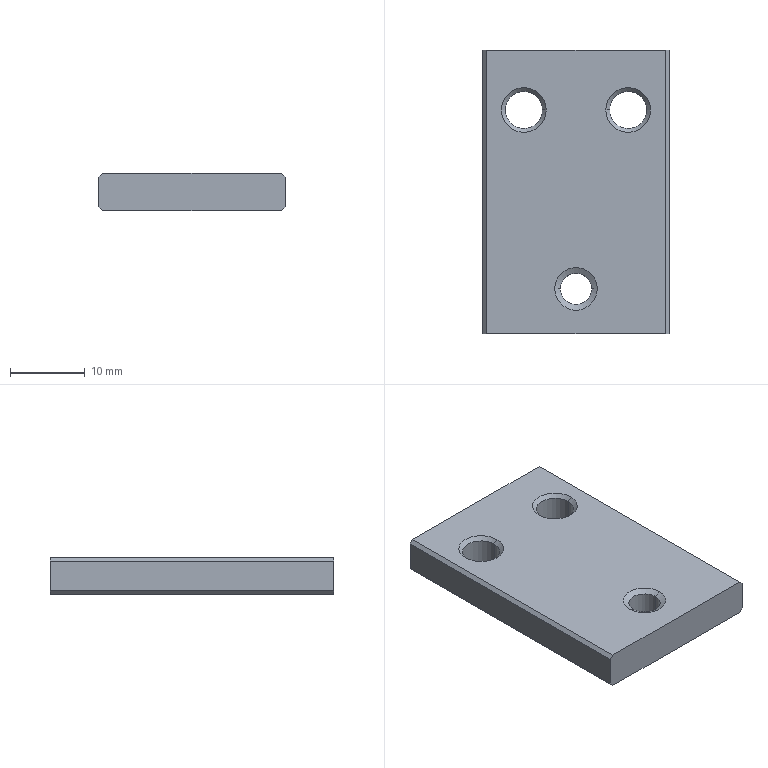Part | NX | 1 solid | 26 faces | box 25 x 38 x 5 mm | volume 4455 mm3 | plane 10 | cone 10 | cylinder 6 | commonest cylinder face diameters 5 x4 4.2 x2
STEP:
#1=CARTESIAN_POINT('',(-12.,-17.53,-2.5));
#2=VERTEX_POINT('',#1);
#3=CARTESIAN_POINT('',(12.,-17.53,-2.5));
#4=VERTEX_POINT('',#3);
#5=CARTESIAN_POINT('',(0.,-17.53,-2.5));
#6=DIRECTION('',(1.,0.,0.));
#7=VECTOR('',#6,1000.);
#8=LINE('',#5,#7);
#9=EDGE_CURVE('',#2,#4,#8,.T.);
#10=ORIENTED_EDGE('',*,*,#9,.F.);
#11=CARTESIAN_POINT('',(-12.,20.47,-2.5));
#12=VERTEX_POINT('',#11);
#13=CARTESIAN_POINT('',(-12.,0.,-2.5));
#14=DIRECTION('',(0.,1.,0.));
#15=VECTOR('',#14,1000.);
#16=LINE('',#13,#15);
#17=EDGE_CURVE('',#2,#12,#16,.T.);
#18=ORIENTED_EDGE('',*,*,#17,.T.);
#19=CARTESIAN_POINT('',(12.,20.47,-2.5));
#20=VERTEX_POINT('',#19);
#21=CARTESIAN_POINT('',(0.,20.47,-2.5));
#22=DIRECTION('',(1.,0.,0.));
#23=VECTOR('',#22,1000.);
#24=LINE('',#21,#23);
#25=EDGE_CURVE('',#12,#20,#24,.T.);
#26=ORIENTED_EDGE('',*,*,#25,.T.);
#27=CARTESIAN_POINT('',(12.,0.,-2.5));
#28=DIRECTION('',(0.,-1.,0.));
#29=VECTOR('',#28,1000.);
#30=LINE('',#27,#29);
#31=EDGE_CURVE('',#20,#4,#30,.T.);
#32=ORIENTED_EDGE('',*,*,#31,.T.);
#33=EDGE_LOOP('',(#10,#18,#26,#32));
#34=FACE_BOUND('',#33,.T.);
#35=CARTESIAN_POINT('',(-4.,12.47,-2.5));
#36=VERTEX_POINT('',#35);
#37=CARTESIAN_POINT('',(-10.,12.47,-2.5));
#38=VERTEX_POINT('',#37);
#39=CARTESIAN_POINT('',(-7.,12.47,-2.5));
#40=DIRECTION('',(0.,0.,-1.));
#41=DIRECTION('',(-1.,0.,0.));
#42=AXIS2_PLACEMENT_3D('',#39,#40,#41);
#43=CIRCLE('',#42,3.);
#44=EDGE_CURVE('',#36,#38,#43,.T.);
#45=ORIENTED_EDGE('',*,*,#44,.F.);
#46=CARTESIAN_POINT('',(-7.,12.47,-2.5));
#47=DIRECTION('',(0.,0.,-1.));
#48=DIRECTION('',(-1.,0.,0.));
#49=AXIS2_PLACEMENT_3D('',#46,#47,#48);
#50=CIRCLE('',#49,3.);
#51=EDGE_CURVE('',#38,#36,#50,.T.);
#52=ORIENTED_EDGE('',*,*,#51,.F.);
#53=EDGE_LOOP('',(#45,#52));
#54=FACE_BOUND('',#53,.T.);
#55=CARTESIAN_POINT('',(10.,12.47,-2.5));
#56=VERTEX_POINT('',#55);
#57=CARTESIAN_POINT('',(4.,12.47,-2.5));
#58=VERTEX_POINT('',#57);
#59=CARTESIAN_POINT('',(7.,12.47,-2.5));
#60=DIRECTION('',(0.,0.,-1.));
#61=DIRECTION('',(-1.,0.,0.));
#62=AXIS2_PLACEMENT_3D('',#59,#60,#61);
#63=CIRCLE('',#62,3.);
#64=EDGE_CURVE('',#56,#58,#63,.T.);
#65=ORIENTED_EDGE('',*,*,#64,.F.);
#66=CARTESIAN_POINT('',(7.,12.47,-2.5));
#67=DIRECTION('',(0.,0.,-1.));
#68=DIRECTION('',(-1.,0.,0.));
#69=AXIS2_PLACEMENT_3D('',#66,#67,#68);
#70=CIRCLE('',#69,3.);
#71=EDGE_CURVE('',#58,#56,#70,.T.);
#72=ORIENTED_EDGE('',*,*,#71,.F.);
#73=EDGE_LOOP('',(#65,#72));
#74=FACE_BOUND('',#73,.T.);
#75=CARTESIAN_POINT('',(2.1,-11.53,-2.5));
#76=VERTEX_POINT('',#75);
#77=CARTESIAN_POINT('',(-2.1,-11.53,-2.5));
#78=VERTEX_POINT('',#77);
#79=CARTESIAN_POINT('',(0.,-11.53,-2.5));
#80=DIRECTION('',(0.,0.,1.));
#81=DIRECTION('',(1.,0.,0.));
#82=AXIS2_PLACEMENT_3D('',#79,#80,#81);
#83=CIRCLE('',#82,2.1);
#84=EDGE_CURVE('',#76,#78,#83,.T.);
#85=ORIENTED_EDGE('',*,*,#84,.T.);
#86=CARTESIAN_POINT('',(0.,-11.53,-2.5));
#87=DIRECTION('',(0.,0.,1.));
#88=DIRECTION('',(1.,0.,0.));
#89=AXIS2_PLACEMENT_3D('',#86,#87,#88);
#90=CIRCLE('',#89,2.1);
#91=EDGE_CURVE('',#78,#76,#90,.T.);
#92=ORIENTED_EDGE('',*,*,#91,.T.);
#93=EDGE_LOOP('',(#85,#92));
#94=FACE_BOUND('',#93,.T.);
#95=CARTESIAN_POINT('',(0.,0.,-2.5));
#96=DIRECTION('',(0.,0.,1.));
#97=DIRECTION('',(1.,0.,0.));
#98=AXIS2_PLACEMENT_3D('',#95,#96,#97);
#99=PLANE('',#98);
#100=ADVANCED_FACE('',(#34,#54,#74,#94),#99,.F.);
#101=CARTESIAN_POINT('',(2.1,-11.53,2.061));
#102=VERTEX_POINT('',#101);
#103=CARTESIAN_POINT('',(-2.1,-11.53,2.061));
#104=VERTEX_POINT('',#103);
#105=CARTESIAN_POINT('',(0.,-11.53,2.061));
#106=DIRECTION('',(0.,0.,1.));
#107=DIRECTION('',(1.,0.,0.));
#108=AXIS2_PLACEMENT_3D('',#105,#106,#107);
#109=CIRCLE('',#108,2.1);
#110=EDGE_CURVE('',#102,#104,#109,.T.);
#111=ORIENTED_EDGE('',*,*,#110,.F.);
#112=CARTESIAN_POINT('',(2.86,-11.53,2.5));
#113=VERTEX_POINT('',#112);
#114=CARTESIAN_POINT('',(2.1,-11.53,2.061));
#115=DIRECTION('',(0.866,0.,0.5));
#116=VECTOR('',#115,1000.);
#117=LINE('',#114,#116);
#118=EDGE_CURVE('',#102,#113,#117,.T.);
#119=ORIENTED_EDGE('',*,*,#118,.T.);
#120=CARTESIAN_POINT('',(-2.86,-11.53,2.5));
#121=VERTEX_POINT('',#120);
#122=CARTESIAN_POINT('',(0.,-11.53,2.5));
#123=DIRECTION('',(0.,0.,1.));
#124=DIRECTION('',(1.,0.,0.));
#125=AXIS2_PLACEMENT_3D('',#122,#123,#124);
#126=CIRCLE('',#125,2.86);
#127=EDGE_CURVE('',#113,#121,#126,.T.);
#128=ORIENTED_EDGE('',*,*,#127,.T.);
#129=CARTESIAN_POINT('',(-2.1,-11.53,2.061));
#130=DIRECTION('',(-0.866,0.,0.5));
#131=VECTOR('',#130,1000.);
#132=LINE('',#129,#131);
#133=EDGE_CURVE('',#104,#121,#132,.T.);
#134=ORIENTED_EDGE('',*,*,#133,.F.);
#135=EDGE_LOOP('',(#111,#119,#128,#134));
#136=FACE_BOUND('',#135,.T.);
#137=CARTESIAN_POINT('',(0.,-11.53,2.061));
#138=DIRECTION('',(0.,0.,1.));
#139=DIRECTION('',(1.,0.,0.));
#140=AXIS2_PLACEMENT_3D('',#137,#138,#139);
#141=CONICAL_SURFACE('',#140,2.1,1.047);
#142=ADVANCED_FACE('',(#136),#141,.F.);
#143=ORIENTED_EDGE('',*,*,#25,.F.);
#144=CARTESIAN_POINT('',(-12.5,20.47,-2.));
#145=VERTEX_POINT('',#144);
#146=CARTESIAN_POINT('',(-14.5,20.47,0.));
#147=DIRECTION('',(-0.7071,0.,0.7071));
#148=VECTOR('',#147,1000.);
#149=LINE('',#146,#148);
#150=EDGE_CURVE('',#12,#145,#149,.T.);
#151=ORIENTED_EDGE('',*,*,#150,.T.);
#152=CARTESIAN_POINT('',(-12.5,20.47,2.));
#153=VERTEX_POINT('',#152);
#154=CARTESIAN_POINT('',(-12.5,20.47,0.));
#155=DIRECTION('',(0.,0.,1.));
#156=VECTOR('',#155,1000.);
#157=LINE('',#154,#156);
#158=EDGE_CURVE('',#145,#153,#157,.T.);
#159=ORIENTED_EDGE('',*,*,#158,.T.);
#160=CARTESIAN_POINT('',(-12.,20.47,2.5));
#161=VERTEX_POINT('',#160);
#162=CARTESIAN_POINT('',(-14.5,20.47,0.));
#163=DIRECTION('',(0.7071,0.,0.7071));
#164=VECTOR('',#163,1000.);
#165=LINE('',#162,#164);
#166=EDGE_CURVE('',#153,#161,#165,.T.);
#167=ORIENTED_EDGE('',*,*,#166,.T.);
#168=CARTESIAN_POINT('',(12.,20.47,2.5));
#169=VERTEX_POINT('',#168);
#170=CARTESIAN_POINT('',(0.,20.47,2.5));
#171=DIRECTION('',(1.,0.,0.));
#172=VECTOR('',#171,1000.);
#173=LINE('',#170,#172);
#174=EDGE_CURVE('',#161,#169,#173,.T.);
#175=ORIENTED_EDGE('',*,*,#174,.T.);
#176=CARTESIAN_POINT('',(12.5,20.47,2.));
#177=VERTEX_POINT('',#176);
#178=CARTESIAN_POINT('',(14.5,20.47,0.));
#179=DIRECTION('',(0.7071,0.,-0.7071));
#180=VECTOR('',#179,1000.);
#181=LINE('',#178,#180);
#182=EDGE_CURVE('',#169,#177,#181,.T.);
#183=ORIENTED_EDGE('',*,*,#182,.T.);
#184=CARTESIAN_POINT('',(12.5,20.47,-2.));
#185=VERTEX_POINT('',#184);
#186=CARTESIAN_POINT('',(12.5,20.47,0.));
#187=DIRECTION('',(0.,0.,-1.));
#188=VECTOR('',#187,1000.);
#189=LINE('',#186,#188);
#190=EDGE_CURVE('',#177,#185,#189,.T.);
#191=ORIENTED_EDGE('',*,*,#190,.T.);
#192=CARTESIAN_POINT('',(14.5,20.47,0.));
#193=DIRECTION('',(-0.7071,0.,-0.7071));
#194=VECTOR('',#193,1000.);
#195=LINE('',#192,#194);
#196=EDGE_CURVE('',#185,#20,#195,.T.);
#197=ORIENTED_EDGE('',*,*,#196,.T.);
#198=EDGE_LOOP('',(#143,#151,#159,#167,#175,#183,#191,#197));
#199=FACE_BOUND('',#198,.T.);
#200=CARTESIAN_POINT('',(-38.,20.47,-99.5));
#201=DIRECTION('',(0.,1.,0.));
#202=DIRECTION('',(1.,0.,0.));
#203=AXIS2_PLACEMENT_3D('',#200,#201,#202);
#204=PLANE('',#203);
#205=ADVANCED_FACE('',(#199),#204,.T.);
#206=CARTESIAN_POINT('',(12.5,-17.53,2.));
#207=VERTEX_POINT('',#206);
#208=CARTESIAN_POINT('',(12.5,0.,2.));
#209=DIRECTION('',(0.,1.,0.));
#210=VECTOR('',#209,1000.);
#211=LINE('',#208,#210);
#212=EDGE_CURVE('',#207,#177,#211,.T.);
#213=ORIENTED_EDGE('',*,*,#212,.F.);
#214=CARTESIAN_POINT('',(12.5,-17.53,-2.));
#215=VERTEX_POINT('',#214);
#216=CARTESIAN_POINT('',(12.5,-17.53,0.));
#217=DIRECTION('',(0.,0.,-1.));
#218=VECTOR('',#217,1000.);
#219=LINE('',#216,#218);
#220=EDGE_CURVE('',#207,#215,#219,.T.);
#221=ORIENTED_EDGE('',*,*,#220,.T.);
#222=CARTESIAN_POINT('',(12.5,0.,-2.));
#223=DIRECTION('',(0.,-1.,0.));
#224=VECTOR('',#223,1000.);
#225=LINE('',#222,#224);
#226=EDGE_CURVE('',#185,#215,#225,.T.);
#227=ORIENTED_EDGE('',*,*,#226,.F.);
#228=ORIENTED_EDGE('',*,*,#190,.F.);
#229=EDGE_LOOP('',(#213,#221,#227,#228));
#230=FACE_BOUND('',#229,.T.);
#231=CARTESIAN_POINT('',(12.5,-20.5,-2.5));
#232=DIRECTION('',(1.,0.,0.));
#233=DIRECTION('',(0.,1.,0.));
#234=AXIS2_PLACEMENT_3D('',#231,#232,#233);
#235=PLANE('',#234);
#236=ADVANCED_FACE('',(#230),#235,.T.);
#237=CARTESIAN_POINT('',(14.5,-17.53,0.));
#238=DIRECTION('',(-0.7071,0.,-0.7071));
#239=VECTOR('',#238,1000.);
#240=LINE('',#237,#239);
#241=EDGE_CURVE('',#215,#4,#240,.T.);
#242=ORIENTED_EDGE('',*,*,#241,.T.);
#243=ORIENTED_EDGE('',*,*,#31,.F.);
#244=ORIENTED_EDGE('',*,*,#196,.F.);
#245=ORIENTED_EDGE('',*,*,#226,.T.);
#246=EDGE_LOOP('',(#242,#243,#244,#245));
#247=FACE_BOUND('',#246,.T.);
#248=CARTESIAN_POINT('',(12.25,0.,-2.25));
#249=DIRECTION('',(0.7071,0.,-0.7071));
#250=DIRECTION('',(0.,-1.,0.));
#251=AXIS2_PLACEMENT_3D('',#248,#249,#250);
#252=PLANE('',#251);
#253=ADVANCED_FACE('',(#247),#252,.T.);
#254=CARTESIAN_POINT('',(-12.5,-17.53,2.));
#255=VERTEX_POINT('',#254);
#256=CARTESIAN_POINT('',(-12.,-17.53,2.5));
#257=VERTEX_POINT('',#256);
#258=CARTESIAN_POINT('',(-14.5,-17.53,0.));
#259=DIRECTION('',(0.7071,0.,0.7071));
#260=VECTOR('',#259,1000.);
#261=LINE('',#258,#260);
#262=EDGE_CURVE('',#255,#257,#261,.T.);
#263=ORIENTED_EDGE('',*,*,#262,.T.);
#264=CARTESIAN_POINT('',(-12.,0.,2.5));
#265=DIRECTION('',(0.,1.,0.));
#266=VECTOR('',#265,1000.);
#267=LINE('',#264,#266);
#268=EDGE_CURVE('',#257,#161,#267,.T.);
#269=ORIENTED_EDGE('',*,*,#268,.T.);
#270=ORIENTED_EDGE('',*,*,#166,.F.);
#271=CARTESIAN_POINT('',(-12.5,0.,2.));
#272=DIRECTION('',(0.,-1.,0.));
#273=VECTOR('',#272,1000.);
#274=LINE('',#271,#273);
#275=EDGE_CURVE('',#153,#255,#274,.T.);
#276=ORIENTED_EDGE('',*,*,#275,.T.);
#277=EDGE_LOOP('',(#263,#269,#270,#276));
#278=FACE_BOUND('',#277,.T.);
#279=CARTESIAN_POINT('',(-12.25,0.,2.25));
#280=DIRECTION('',(-0.7071,0.,0.7071));
#281=DIRECTION('',(0.,1.,0.));
#282=AXIS2_PLACEMENT_3D('',#279,#280,#281);
#283=PLANE('',#282);
#284=ADVANCED_FACE('',(#278),#283,.T.);
#285=CARTESIAN_POINT('',(-4.5,12.47,2.));
#286=VERTEX_POINT('',#285);
#287=CARTESIAN_POINT('',(-9.5,12.47,2.));
#288=VERTEX_POINT('',#287);
#289=CARTESIAN_POINT('',(-7.,12.47,2.));
#290=DIRECTION('',(0.,0.,-1.));
#291=DIRECTION('',(-1.,0.,0.));
#292=AXIS2_PLACEMENT_3D('',#289,#290,#291);
#293=CIRCLE('',#292,2.5);
#294=EDGE_CURVE('',#286,#288,#293,.T.);
#295=ORIENTED_EDGE('',*,*,#294,.F.);
#296=CARTESIAN_POINT('',(-4.5,12.47,-2.));
#297=VERTEX_POINT('',#296);
#298=CARTESIAN_POINT('',(-4.5,12.47,2.5));
#299=DIRECTION('',(0.,0.,-1.));
#300=VECTOR('',#299,1000.);
#301=LINE('',#298,#300);
#302=EDGE_CURVE('',#286,#297,#301,.T.);
#303=ORIENTED_EDGE('',*,*,#302,.T.);
#304=CARTESIAN_POINT('',(-9.5,12.47,-2.));
#305=VERTEX_POINT('',#304);
#306=CARTESIAN_POINT('',(-7.,12.47,-2.));
#307=DIRECTION('',(0.,0.,-1.));
#308=DIRECTION('',(-1.,0.,0.));
#309=AXIS2_PLACEMENT_3D('',#306,#307,#308);
#310=CIRCLE('',#309,2.5);
#311=EDGE_CURVE('',#297,#305,#310,.T.);
#312=ORIENTED_EDGE('',*,*,#311,.T.);
#313=CARTESIAN_POINT('',(-9.5,12.47,2.5));
#314=DIRECTION('',(0.,0.,-1.));
#315=VECTOR('',#314,1000.);
#316=LINE('',#313,#315);
#317=EDGE_CURVE('',#288,#305,#316,.T.);
#318=ORIENTED_EDGE('',*,*,#317,.F.);
#319=EDGE_LOOP('',(#295,#303,#312,#318));
#320=FACE_BOUND('',#319,.T.);
#321=CARTESIAN_POINT('',(-7.,12.47,2.5));
#322=DIRECTION('',(0.,0.,-1.));
#323=DIRECTION('',(-1.,0.,0.));
#324=AXIS2_PLACEMENT_3D('',#321,#322,#323);
#325=CYLINDRICAL_SURFACE('',#324,2.5);
#326=ADVANCED_FACE('',(#320),#325,.F.);
#327=CARTESIAN_POINT('',(9.5,12.47,-2.));
#328=VERTEX_POINT('',#327);
#329=CARTESIAN_POINT('',(4.5,12.47,-2.));
#330=VERTEX_POINT('',#329);
#331=CARTESIAN_POINT('',(7.,12.47,-2.));
#332=DIRECTION('',(0.,0.,-1.));
#333=DIRECTION('',(-1.,0.,0.));
#334=AXIS2_PLACEMENT_3D('',#331,#332,#333);
#335=CIRCLE('',#334,2.5);
#336=EDGE_CURVE('',#328,#330,#335,.T.);
#337=ORIENTED_EDGE('',*,*,#336,.T.);
#338=CARTESIAN_POINT('',(4.5,12.47,2.));
#339=VERTEX_POINT('',#338);
#340=CARTESIAN_POINT('',(4.5,12.47,2.5));
#341=DIRECTION('',(0.,0.,-1.));
#342=VECTOR('',#341,1000.);
#343=LINE('',#340,#342);
#344=EDGE_CURVE('',#330,#339,#343,.F.);
#345=ORIENTED_EDGE('',*,*,#344,.T.);
#346=CARTESIAN_POINT('',(9.5,12.47,2.));
#347=VERTEX_POINT('',#346);
#348=CARTESIAN_POINT('',(7.,12.47,2.));
#349=DIRECTION('',(0.,0.,-1.));
#350=DIRECTION('',(-1.,0.,0.));
#351=AXIS2_PLACEMENT_3D('',#348,#349,#350);
#352=CIRCLE('',#351,2.5);
#353=EDGE_CURVE('',#347,#339,#352,.T.);
#354=ORIENTED_EDGE('',*,*,#353,.F.);
#355=CARTESIAN_POINT('',(9.5,12.47,2.5));
#356=DIRECTION('',(0.,0.,-1.));
#357=VECTOR('',#356,1000.);
#358=LINE('',#355,#357);
#359=EDGE_CURVE('',#328,#347,#358,.F.);
#360=ORIENTED_EDGE('',*,*,#359,.F.);
#361=EDGE_LOOP('',(#337,#345,#354,#360));
#362=FACE_BOUND('',#361,.T.);
#363=CARTESIAN_POINT('',(7.,12.47,2.5));
#364=DIRECTION('',(0.,0.,-1.));
#365=DIRECTION('',(-1.,0.,0.));
#366=AXIS2_PLACEMENT_3D('',#363,#364,#365);
#367=CYLINDRICAL_SURFACE('',#366,2.5);
#368=ADVANCED_FACE('',(#362),#367,.F.);
#369=ORIENTED_EDGE('',*,*,#212,.T.);
#370=ORIENTED_EDGE('',*,*,#182,.F.);
#371=CARTESIAN_POINT('',(12.,-17.53,2.5));
#372=VERTEX_POINT('',#371);
#373=CARTESIAN_POINT('',(12.,0.,2.5));
#374=DIRECTION('',(0.,-1.,0.));
#375=VECTOR('',#374,1000.);
#376=LINE('',#373,#375);
#377=EDGE_CURVE('',#169,#372,#376,.T.);
#378=ORIENTED_EDGE('',*,*,#377,.T.);
#379=CARTESIAN_POINT('',(14.5,-17.53,0.));
#380=DIRECTION('',(0.7071,0.,-0.7071));
#381=VECTOR('',#380,1000.);
#382=LINE('',#379,#381);
#383=EDGE_CURVE('',#372,#207,#382,.T.);
#384=ORIENTED_EDGE('',*,*,#383,.T.);
#385=EDGE_LOOP('',(#369,#370,#378,#384));
#386=FACE_BOUND('',#385,.T.);
#387=CARTESIAN_POINT('',(12.25,0.,2.25));
#388=DIRECTION('',(0.7071,0.,0.7071));
#389=DIRECTION('',(0.,-1.,0.));
#390=AXIS2_PLACEMENT_3D('',#387,#388,#389);
#391=PLANE('',#390);
#392=ADVANCED_FACE('',(#386),#391,.T.);
#393=CARTESIAN_POINT('',(-12.5,-17.53,-2.));
#394=VERTEX_POINT('',#393);
#395=CARTESIAN_POINT('',(-12.5,-17.53,0.));
#396=DIRECTION('',(0.,0.,1.));
#397=VECTOR('',#396,1000.);
#398=LINE('',#395,#397);
#399=EDGE_CURVE('',#394,#255,#398,.T.);
#400=ORIENTED_EDGE('',*,*,#399,.T.);
#401=ORIENTED_EDGE('',*,*,#275,.F.);
#402=ORIENTED_EDGE('',*,*,#158,.F.);
#403=CARTESIAN_POINT('',(-12.5,0.,-2.));
#404=DIRECTION('',(0.,1.,0.));
#405=VECTOR('',#404,1000.);
#406=LINE('',#403,#405);
#407=EDGE_CURVE('',#394,#145,#406,.T.);
#408=ORIENTED_EDGE('',*,*,#407,.F.);
#409=EDGE_LOOP('',(#400,#401,#402,#408));
#410=FACE_BOUND('',#409,.T.);
#411=CARTESIAN_POINT('',(-12.5,20.5,-2.5));
#412=DIRECTION('',(-1.,0.,0.));
#413=DIRECTION('',(0.,0.,1.));
#414=AXIS2_PLACEMENT_3D('',#411,#412,#413);
#415=PLANE('',#414);
#416=ADVANCED_FACE('',(#410),#415,.T.);
#417=CARTESIAN_POINT('',(-10.,12.47,2.5));
#418=VERTEX_POINT('',#417);
#419=CARTESIAN_POINT('',(-4.,12.47,2.5));
#420=VERTEX_POINT('',#419);
#421=CARTESIAN_POINT('',(-7.,12.47,2.5));
#422=DIRECTION('',(0.,0.,1.));
#423=DIRECTION('',(1.,0.,0.));
#424=AXIS2_PLACEMENT_3D('',#421,#422,#423);
#425=CIRCLE('',#424,3.);
#426=EDGE_CURVE('',#418,#420,#425,.T.);
#427=ORIENTED_EDGE('',*,*,#426,.T.);
#428=CARTESIAN_POINT('',(-4.,12.47,2.5));
#429=DIRECTION('',(0.7071,0.,0.7071));
#430=VECTOR('',#429,1000.);
#431=LINE('',#428,#430);
#432=EDGE_CURVE('',#286,#420,#431,.T.);
#433=ORIENTED_EDGE('',*,*,#432,.F.);
#434=ORIENTED_EDGE('',*,*,#294,.T.);
#435=CARTESIAN_POINT('',(-10.,12.47,2.5));
#436=DIRECTION('',(-0.7071,0.,0.7071));
#437=VECTOR('',#436,1000.);
#438=LINE('',#435,#437);
#439=EDGE_CURVE('',#288,#418,#438,.T.);
#440=ORIENTED_EDGE('',*,*,#439,.T.);
#441=EDGE_LOOP('',(#427,#433,#434,#440));
#442=FACE_BOUND('',#441,.T.);
#443=CARTESIAN_POINT('',(-7.,12.47,2.5));
#444=DIRECTION('',(0.,0.,1.));
#445=DIRECTION('',(1.,0.,0.));
#446=AXIS2_PLACEMENT_3D('',#443,#444,#445);
#447=CONICAL_SURFACE('',#446,3.,0.7854);
#448=ADVANCED_FACE('',(#442),#447,.F.);
#449=ORIENTED_EDGE('',*,*,#353,.T.);
#450=CARTESIAN_POINT('',(4.,12.47,2.5));
#451=VERTEX_POINT('',#450);
#452=CARTESIAN_POINT('',(4.,12.47,2.5));
#453=DIRECTION('',(-0.7071,0.,0.7071));
#454=VECTOR('',#453,1000.);
#455=LINE('',#452,#454);
#456=EDGE_CURVE('',#339,#451,#455,.T.);
#457=ORIENTED_EDGE('',*,*,#456,.T.);
#458=CARTESIAN_POINT('',(10.,12.47,2.5));
#459=VERTEX_POINT('',#458);
#460=CARTESIAN_POINT('',(7.,12.47,2.5));
#461=DIRECTION('',(0.,0.,1.));
#462=DIRECTION('',(1.,0.,0.));
#463=AXIS2_PLACEMENT_3D('',#460,#461,#462);
#464=CIRCLE('',#463,3.);
#465=EDGE_CURVE('',#451,#459,#464,.T.);
#466=ORIENTED_EDGE('',*,*,#465,.T.);
#467=CARTESIAN_POINT('',(10.,12.47,2.5));
#468=DIRECTION('',(0.7071,0.,0.7071));
#469=VECTOR('',#468,1000.);
#470=LINE('',#467,#469);
#471=EDGE_CURVE('',#347,#459,#470,.T.);
#472=ORIENTED_EDGE('',*,*,#471,.F.);
#473=EDGE_LOOP('',(#449,#457,#466,#472));
#474=FACE_BOUND('',#473,.T.);
#475=CARTESIAN_POINT('',(7.,12.47,2.5));
#476=DIRECTION('',(0.,0.,1.));
#477=DIRECTION('',(1.,0.,0.));
#478=AXIS2_PLACEMENT_3D('',#475,#476,#477);
#479=CONICAL_SURFACE('',#478,3.,0.7854);
#480=ADVANCED_FACE('',(#474),#479,.F.);
#481=ORIENTED_EDGE('',*,*,#64,.T.);
#482=CARTESIAN_POINT('',(4.,12.47,-2.5));
#483=DIRECTION('',(-0.7071,0.,-0.7071));
#484=VECTOR('',#483,1000.);
#485=LINE('',#482,#484);
#486=EDGE_CURVE('',#58,#330,#485,.F.);
#487=ORIENTED_EDGE('',*,*,#486,.T.);
#488=ORIENTED_EDGE('',*,*,#336,.F.);
#489=CARTESIAN_POINT('',(10.,12.47,-2.5));
#490=DIRECTION('',(0.7071,0.,-0.7071));
#491=VECTOR('',#490,1000.);
#492=LINE('',#489,#491);
#493=EDGE_CURVE('',#56,#328,#492,.F.);
#494=ORIENTED_EDGE('',*,*,#493,.F.);
#495=EDGE_LOOP('',(#481,#487,#488,#494));
#496=FACE_BOUND('',#495,.T.);
#497=CARTESIAN_POINT('',(7.,12.47,-2.5));
#498=DIRECTION('',(0.,0.,-1.));
#499=DIRECTION('',(-1.,0.,0.));
#500=AXIS2_PLACEMENT_3D('',#497,#498,#499);
#501=CONICAL_SURFACE('',#500,3.,0.7854);
#502=ADVANCED_FACE('',(#496),#501,.F.);
#503=ORIENTED_EDGE('',*,*,#44,.T.);
#504=CARTESIAN_POINT('',(-10.,12.47,-2.5));
#505=DIRECTION('',(-0.7071,0.,-0.7071));
#506=VECTOR('',#505,1000.);
#507=LINE('',#504,#506);
#508=EDGE_CURVE('',#38,#305,#507,.F.);
#509=ORIENTED_EDGE('',*,*,#508,.T.);
#510=ORIENTED_EDGE('',*,*,#311,.F.);
#511=CARTESIAN_POINT('',(-4.,12.47,-2.5));
#512=DIRECTION('',(0.7071,0.,-0.7071));
#513=VECTOR('',#512,1000.);
#514=LINE('',#511,#513);
#515=EDGE_CURVE('',#36,#297,#514,.F.);
#516=ORIENTED_EDGE('',*,*,#515,.F.);
#517=EDGE_LOOP('',(#503,#509,#510,#516));
#518=FACE_BOUND('',#517,.T.);
#519=CARTESIAN_POINT('',(-7.,12.47,-2.5));
#520=DIRECTION('',(0.,0.,-1.));
#521=DIRECTION('',(-1.,0.,0.));
#522=AXIS2_PLACEMENT_3D('',#519,#520,#521);
#523=CONICAL_SURFACE('',#522,3.,0.7854);
#524=ADVANCED_FACE('',(#518),#523,.F.);
#525=ORIENTED_EDGE('',*,*,#17,.F.);
#526=CARTESIAN_POINT('',(-14.5,-17.53,0.));
#527=DIRECTION('',(0.7071,0.,-0.7071));
#528=VECTOR('',#527,1000.);
#529=LINE('',#526,#528);
#530=EDGE_CURVE('',#394,#2,#529,.T.);
#531=ORIENTED_EDGE('',*,*,#530,.F.);
#532=ORIENTED_EDGE('',*,*,#407,.T.);
#533=ORIENTED_EDGE('',*,*,#150,.F.);
#534=EDGE_LOOP('',(#525,#531,#532,#533));
#535=FACE_BOUND('',#534,.T.);
#536=CARTESIAN_POINT('',(-12.25,0.,-2.25));
#537=DIRECTION('',(-0.7071,0.,-0.7071));
#538=DIRECTION('',(-0.7071,0.,0.7071));
#539=AXIS2_PLACEMENT_3D('',#536,#537,#538);
#540=PLANE('',#539);
#541=ADVANCED_FACE('',(#535),#540,.T.);
#542=ORIENTED_EDGE('',*,*,#268,.F.);
#543=CARTESIAN_POINT('',(0.,-17.53,2.5));
#544=DIRECTION('',(1.,0.,0.));
#545=VECTOR('',#544,1000.);
#546=LINE('',#543,#545);
#547=EDGE_CURVE('',#257,#372,#546,.T.);
#548=ORIENTED_EDGE('',*,*,#547,.T.);
#549=ORIENTED_EDGE('',*,*,#377,.F.);
#550=ORIENTED_EDGE('',*,*,#174,.F.);
#551=EDGE_LOOP('',(#542,#548,#549,#550));
#552=FACE_BOUND('',#551,.T.);
#553=ORIENTED_EDGE('',*,*,#426,.F.);
#554=CARTESIAN_POINT('',(-7.,12.47,2.5));
#555=DIRECTION('',(0.,0.,1.));
#556=DIRECTION('',(1.,0.,0.));
#557=AXIS2_PLACEMENT_3D('',#554,#555,#556);
#558=CIRCLE('',#557,3.);
#559=EDGE_CURVE('',#420,#418,#558,.T.);
#560=ORIENTED_EDGE('',*,*,#559,.F.);
#561=EDGE_LOOP('',(#553,#560));
#562=FACE_BOUND('',#561,.T.);
#563=CARTESIAN_POINT('',(0.,-11.53,2.5));
#564=DIRECTION('',(0.,0.,1.));
#565=DIRECTION('',(1.,0.,0.));
#566=AXIS2_PLACEMENT_3D('',#563,#564,#565);
#567=CIRCLE('',#566,2.86);
#568=EDGE_CURVE('',#121,#113,#567,.T.);
#569=ORIENTED_EDGE('',*,*,#568,.F.);
#570=ORIENTED_EDGE('',*,*,#127,.F.);
#571=EDGE_LOOP('',(#569,#570));
#572=FACE_BOUND('',#571,.T.);
#573=ORIENTED_EDGE('',*,*,#465,.F.);
#574=CARTESIAN_POINT('',(7.,12.47,2.5));
#575=DIRECTION('',(0.,0.,1.));
#576=DIRECTION('',(1.,0.,0.));
#577=AXIS2_PLACEMENT_3D('',#574,#575,#576);
#578=CIRCLE('',#577,3.);
#579=EDGE_CURVE('',#459,#451,#578,.T.);
#580=ORIENTED_EDGE('',*,*,#579,.F.);
#581=EDGE_LOOP('',(#573,#580));
#582=FACE_BOUND('',#581,.T.);
#583=CARTESIAN_POINT('',(0.,0.,2.5));
#584=DIRECTION('',(0.,0.,1.));
#585=DIRECTION('',(1.,0.,0.));
#586=AXIS2_PLACEMENT_3D('',#583,#584,#585);
#587=PLANE('',#586);
#588=ADVANCED_FACE('',(#552,#562,#572,#582),#587,.T.);
#589=ORIENTED_EDGE('',*,*,#110,.T.);
#590=CARTESIAN_POINT('',(-2.1,-11.53,2.5));
#591=DIRECTION('',(0.,0.,1.));
#592=VECTOR('',#591,1000.);
#593=LINE('',#590,#592);
#594=EDGE_CURVE('',#78,#104,#593,.T.);
#595=ORIENTED_EDGE('',*,*,#594,.F.);
#596=ORIENTED_EDGE('',*,*,#84,.F.);
#597=CARTESIAN_POINT('',(2.1,-11.53,2.5));
#598=DIRECTION('',(0.,0.,1.));
#599=VECTOR('',#598,1000.);
#600=LINE('',#597,#599);
#601=EDGE_CURVE('',#76,#102,#600,.T.);
#602=ORIENTED_EDGE('',*,*,#601,.T.);
#603=EDGE_LOOP('',(#589,#595,#596,#602));
#604=FACE_BOUND('',#603,.T.);
#605=CARTESIAN_POINT('',(0.,-11.53,2.5));
#606=DIRECTION('',(0.,0.,1.));
#607=DIRECTION('',(1.,0.,0.));
#608=AXIS2_PLACEMENT_3D('',#605,#606,#607);
#609=CYLINDRICAL_SURFACE('',#608,2.1);
#610=ADVANCED_FACE('',(#604),#609,.F.);
#611=ORIENTED_EDGE('',*,*,#547,.F.);
#612=ORIENTED_EDGE('',*,*,#262,.F.);
#613=ORIENTED_EDGE('',*,*,#399,.F.);
#614=ORIENTED_EDGE('',*,*,#530,.T.);
#615=ORIENTED_EDGE('',*,*,#9,.T.);
#616=ORIENTED_EDGE('',*,*,#241,.F.);
#617=ORIENTED_EDGE('',*,*,#220,.F.);
#618=ORIENTED_EDGE('',*,*,#383,.F.);
#619=EDGE_LOOP('',(#611,#612,#613,#614,#615,#616,#617,#618));
#620=FACE_BOUND('',#619,.T.);
#621=CARTESIAN_POINT('',(179.5,-17.53,3.));
#622=DIRECTION('',(0.,1.,0.));
#623=DIRECTION('',(1.,0.,0.));
#624=AXIS2_PLACEMENT_3D('',#621,#622,#623);
#625=PLANE('',#624);
#626=ADVANCED_FACE('',(#620),#625,.F.);
#627=CARTESIAN_POINT('',(-7.,12.47,-2.));
#628=DIRECTION('',(0.,0.,-1.));
#629=DIRECTION('',(-1.,0.,0.));
#630=AXIS2_PLACEMENT_3D('',#627,#628,#629);
#631=CIRCLE('',#630,2.5);
#632=EDGE_CURVE('',#305,#297,#631,.T.);
#633=ORIENTED_EDGE('',*,*,#632,.T.);
#634=ORIENTED_EDGE('',*,*,#302,.F.);
#635=CARTESIAN_POINT('',(-7.,12.47,2.));
#636=DIRECTION('',(0.,0.,-1.));
#637=DIRECTION('',(-1.,0.,0.));
#638=AXIS2_PLACEMENT_3D('',#635,#636,#637);
#639=CIRCLE('',#638,2.5);
#640=EDGE_CURVE('',#288,#286,#639,.T.);
#641=ORIENTED_EDGE('',*,*,#640,.F.);
#642=ORIENTED_EDGE('',*,*,#317,.T.);
#643=EDGE_LOOP('',(#633,#634,#641,#642));
#644=FACE_BOUND('',#643,.T.);
#645=CARTESIAN_POINT('',(-7.,12.47,2.5));
#646=DIRECTION('',(0.,0.,-1.));
#647=DIRECTION('',(-1.,0.,0.));
#648=AXIS2_PLACEMENT_3D('',#645,#646,#647);
#649=CYLINDRICAL_SURFACE('',#648,2.5);
#650=ADVANCED_FACE('',(#644),#649,.F.);
#651=ORIENTED_EDGE('',*,*,#486,.F.);
#652=ORIENTED_EDGE('',*,*,#71,.T.);
#653=ORIENTED_EDGE('',*,*,#493,.T.);
#654=CARTESIAN_POINT('',(7.,12.47,-2.));
#655=DIRECTION('',(0.,0.,-1.));
#656=DIRECTION('',(-1.,0.,0.));
#657=AXIS2_PLACEMENT_3D('',#654,#655,#656);
#658=CIRCLE('',#657,2.5);
#659=EDGE_CURVE('',#330,#328,#658,.T.);
#660=ORIENTED_EDGE('',*,*,#659,.F.);
#661=EDGE_LOOP('',(#651,#652,#653,#660));
#662=FACE_BOUND('',#661,.T.);
#663=CARTESIAN_POINT('',(7.,12.47,-2.5));
#664=DIRECTION('',(0.,0.,-1.));
#665=DIRECTION('',(-1.,0.,0.));
#666=AXIS2_PLACEMENT_3D('',#663,#664,#665);
#667=CONICAL_SURFACE('',#666,3.,0.7854);
#668=ADVANCED_FACE('',(#662),#667,.F.);
#669=ORIENTED_EDGE('',*,*,#432,.T.);
#670=ORIENTED_EDGE('',*,*,#559,.T.);
#671=ORIENTED_EDGE('',*,*,#439,.F.);
#672=ORIENTED_EDGE('',*,*,#640,.T.);
#673=EDGE_LOOP('',(#669,#670,#671,#672));
#674=FACE_BOUND('',#673,.T.);
#675=CARTESIAN_POINT('',(-7.,12.47,2.5));
#676=DIRECTION('',(0.,0.,1.));
#677=DIRECTION('',(1.,0.,0.));
#678=AXIS2_PLACEMENT_3D('',#675,#676,#677);
#679=CONICAL_SURFACE('',#678,3.,0.7854);
#680=ADVANCED_FACE('',(#674),#679,.F.);
#681=ORIENTED_EDGE('',*,*,#344,.F.);
#682=ORIENTED_EDGE('',*,*,#659,.T.);
#683=ORIENTED_EDGE('',*,*,#359,.T.);
#684=CARTESIAN_POINT('',(7.,12.47,2.));
#685=DIRECTION('',(0.,0.,-1.));
#686=DIRECTION('',(-1.,0.,0.));
#687=AXIS2_PLACEMENT_3D('',#684,#685,#686);
#688=CIRCLE('',#687,2.5);
#689=EDGE_CURVE('',#339,#347,#688,.T.);
#690=ORIENTED_EDGE('',*,*,#689,.F.);
#691=EDGE_LOOP('',(#681,#682,#683,#690));
#692=FACE_BOUND('',#691,.T.);
#693=CARTESIAN_POINT('',(7.,12.47,2.5));
#694=DIRECTION('',(0.,0.,-1.));
#695=DIRECTION('',(-1.,0.,0.));
#696=AXIS2_PLACEMENT_3D('',#693,#694,#695);
#697=CYLINDRICAL_SURFACE('',#696,2.5);
#698=ADVANCED_FACE('',(#692),#697,.F.);
#699=ORIENTED_EDGE('',*,*,#471,.T.);
#700=ORIENTED_EDGE('',*,*,#579,.T.);
#701=ORIENTED_EDGE('',*,*,#456,.F.);
#702=ORIENTED_EDGE('',*,*,#689,.T.);
#703=EDGE_LOOP('',(#699,#700,#701,#702));
#704=FACE_BOUND('',#703,.T.);
#705=CARTESIAN_POINT('',(7.,12.47,2.5));
#706=DIRECTION('',(0.,0.,1.));
#707=DIRECTION('',(1.,0.,0.));
#708=AXIS2_PLACEMENT_3D('',#705,#706,#707);
#709=CONICAL_SURFACE('',#708,3.,0.7854);
#710=ADVANCED_FACE('',(#704),#709,.F.);
#711=ORIENTED_EDGE('',*,*,#601,.F.);
#712=ORIENTED_EDGE('',*,*,#91,.F.);
#713=ORIENTED_EDGE('',*,*,#594,.T.);
#714=CARTESIAN_POINT('',(0.,-11.53,2.061));
#715=DIRECTION('',(0.,0.,1.));
#716=DIRECTION('',(1.,0.,0.));
#717=AXIS2_PLACEMENT_3D('',#714,#715,#716);
#718=CIRCLE('',#717,2.1);
#719=EDGE_CURVE('',#104,#102,#718,.T.);
#720=ORIENTED_EDGE('',*,*,#719,.T.);
#721=EDGE_LOOP('',(#711,#712,#713,#720));
#722=FACE_BOUND('',#721,.T.);
#723=CARTESIAN_POINT('',(0.,-11.53,2.5));
#724=DIRECTION('',(0.,0.,1.));
#725=DIRECTION('',(1.,0.,0.));
#726=AXIS2_PLACEMENT_3D('',#723,#724,#725);
#727=CYLINDRICAL_SURFACE('',#726,2.1);
#728=ADVANCED_FACE('',(#722),#727,.F.);
#729=ORIENTED_EDGE('',*,*,#568,.T.);
#730=ORIENTED_EDGE('',*,*,#118,.F.);
#731=ORIENTED_EDGE('',*,*,#719,.F.);
#732=ORIENTED_EDGE('',*,*,#133,.T.);
#733=EDGE_LOOP('',(#729,#730,#731,#732));
#734=FACE_BOUND('',#733,.T.);
#735=CARTESIAN_POINT('',(0.,-11.53,2.061));
#736=DIRECTION('',(0.,0.,1.));
#737=DIRECTION('',(1.,0.,0.));
#738=AXIS2_PLACEMENT_3D('',#735,#736,#737);
#739=CONICAL_SURFACE('',#738,2.1,1.047);
#740=ADVANCED_FACE('',(#734),#739,.F.);
#741=ORIENTED_EDGE('',*,*,#632,.F.);
#742=ORIENTED_EDGE('',*,*,#508,.F.);
#743=ORIENTED_EDGE('',*,*,#51,.T.);
#744=ORIENTED_EDGE('',*,*,#515,.T.);
#745=EDGE_LOOP('',(#741,#742,#743,#744));
#746=FACE_BOUND('',#745,.T.);
#747=CARTESIAN_POINT('',(-7.,12.47,-2.5));
#748=DIRECTION('',(0.,0.,-1.));
#749=DIRECTION('',(-1.,0.,0.));
#750=AXIS2_PLACEMENT_3D('',#747,#748,#749);
#751=CONICAL_SURFACE('',#750,3.,0.7854);
#752=ADVANCED_FACE('',(#746),#751,.F.);
#753=CLOSED_SHELL('',(#100,#142,#205,#236,#253,#284,#326,#368,#392,#416,#448,#480,#502,#524,#541,#588,#610,#626,#650,#668,#680,#698,#710,#728,#740,#752));
#754=MANIFOLD_SOLID_BREP('',#753);
#755=(LENGTH_UNIT()NAMED_UNIT(*)SI_UNIT(.MILLI.,.METRE.));
#756=UNCERTAINTY_MEASURE_WITH_UNIT(LENGTH_MEASURE(0.00001),#755,'','');
#757=(NAMED_UNIT(*)PLANE_ANGLE_UNIT()SI_UNIT($,.RADIAN.));
#758=(NAMED_UNIT(*)SI_UNIT($,.STERADIAN.)SOLID_ANGLE_UNIT());
#759=(GEOMETRIC_REPRESENTATION_CONTEXT(3)GLOBAL_UNCERTAINTY_ASSIGNED_CONTEXT((#756))GLOBAL_UNIT_ASSIGNED_CONTEXT((#755,#757,#758))REPRESENTATION_CONTEXT('',''));
#760=ADVANCED_BREP_SHAPE_REPRESENTATION('',(#754),#759);